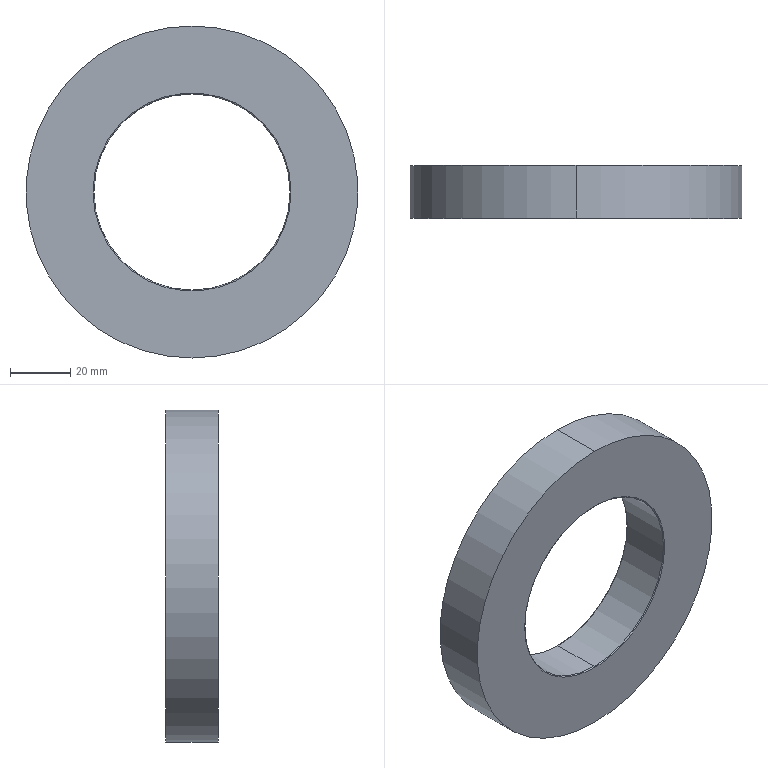Part | SolidWorks | features BaseBody 1 | 1 solid | 10 faces | box 110 x 17.5 x 110 mm | volume 108230 mm3 | cylinder 4 | torus 4 | plane 2 | commonest cylinder face diameters 65 x2 110 x2
STEP:
#1=CARTESIAN_POINT('',(-2100.15,726.569,-1577.624));
#2=VERTEX_POINT('',#1);
#3=CARTESIAN_POINT('',(-2165.75,726.569,-1577.624));
#4=VERTEX_POINT('',#3);
#5=CARTESIAN_POINT('',(-2132.95,726.569,-1577.624));
#6=DIRECTION('',(0.,-1.,0.));
#7=DIRECTION('',(0.,0.,1.));
#8=AXIS2_PLACEMENT_3D('',#5,#6,#7);
#9=CIRCLE('',#8,32.8);
#10=EDGE_CURVE('',#2,#4,#9,.T.);
#11=ORIENTED_EDGE('',*,*,#10,.F.);
#12=CARTESIAN_POINT('',(-2132.95,726.569,-1577.624));
#13=DIRECTION('',(0.,-1.,0.));
#14=DIRECTION('',(-1.,0.,0.));
#15=AXIS2_PLACEMENT_3D('',#12,#13,#14);
#16=CIRCLE('',#15,32.8);
#17=EDGE_CURVE('',#4,#2,#16,.T.);
#18=ORIENTED_EDGE('',*,*,#17,.F.);
#19=EDGE_LOOP('',(#11,#18));
#20=FACE_BOUND('',#19,.T.);
#21=CARTESIAN_POINT('',(-2132.95,726.569,-1522.624));
#22=VERTEX_POINT('',#21);
#23=CARTESIAN_POINT('',(-2132.95,726.569,-1632.624));
#24=VERTEX_POINT('',#23);
#25=CARTESIAN_POINT('',(-2132.95,726.569,-1577.624));
#26=DIRECTION('',(0.,-1.,0.));
#27=DIRECTION('',(0.,0.,1.));
#28=AXIS2_PLACEMENT_3D('',#25,#26,#27);
#29=CIRCLE('',#28,55.);
#30=EDGE_CURVE('',#22,#24,#29,.T.);
#31=ORIENTED_EDGE('',*,*,#30,.T.);
#32=CARTESIAN_POINT('',(-2132.95,726.569,-1577.624));
#33=DIRECTION('',(0.,-1.,0.));
#34=DIRECTION('',(0.,0.,-1.));
#35=AXIS2_PLACEMENT_3D('',#32,#33,#34);
#36=CIRCLE('',#35,55.);
#37=EDGE_CURVE('',#24,#22,#36,.T.);
#38=ORIENTED_EDGE('',*,*,#37,.T.);
#39=EDGE_LOOP('',(#31,#38));
#40=FACE_OUTER_BOUND('',#39,.T.);
#41=CARTESIAN_POINT('',(-2072.49,726.569,-1638.124));
#42=DIRECTION('',(0.,-1.,0.));
#43=DIRECTION('',(0.,0.,-1.));
#44=AXIS2_PLACEMENT_3D('',#41,#42,#43);
#45=PLANE('',#44);
#46=ADVANCED_FACE('',(#20,#40),#45,.T.);
#47=CARTESIAN_POINT('',(-2132.95,744.069,-1522.624));
#48=VERTEX_POINT('',#47);
#49=CARTESIAN_POINT('',(-2132.95,744.069,-1522.624));
#50=DIRECTION('',(0.,-1.,0.));
#51=VECTOR('',#50,1000.);
#52=LINE('',#49,#51);
#53=EDGE_CURVE('',#48,#22,#52,.T.);
#54=ORIENTED_EDGE('',*,*,#53,.T.);
#55=ORIENTED_EDGE('',*,*,#37,.F.);
#56=CARTESIAN_POINT('',(-2132.95,744.069,-1632.624));
#57=VERTEX_POINT('',#56);
#58=CARTESIAN_POINT('',(-2132.95,726.569,-1632.624));
#59=DIRECTION('',(0.,1.,0.));
#60=VECTOR('',#59,1000.);
#61=LINE('',#58,#60);
#62=EDGE_CURVE('',#24,#57,#61,.T.);
#63=ORIENTED_EDGE('',*,*,#62,.T.);
#64=CARTESIAN_POINT('',(-2132.95,744.069,-1577.624));
#65=DIRECTION('',(0.,1.,0.));
#66=DIRECTION('',(0.,0.,1.));
#67=AXIS2_PLACEMENT_3D('',#64,#65,#66);
#68=CIRCLE('',#67,55.);
#69=EDGE_CURVE('',#48,#57,#68,.T.);
#70=ORIENTED_EDGE('',*,*,#69,.F.);
#71=EDGE_LOOP('',(#54,#55,#63,#70));
#72=FACE_OUTER_BOUND('',#71,.T.);
#73=CARTESIAN_POINT('',(-2132.95,744.944,-1577.624));
#74=DIRECTION('',(0.,1.,0.));
#75=DIRECTION('',(-0.08716,0.,0.9962));
#76=AXIS2_PLACEMENT_3D('',#73,#74,#75);
#77=CYLINDRICAL_SURFACE('',#76,55.);
#78=ADVANCED_FACE('',(#72),#77,.T.);
#79=CARTESIAN_POINT('',(-2165.75,744.069,-1577.624));
#80=VERTEX_POINT('',#79);
#81=CARTESIAN_POINT('',(-2100.15,744.069,-1577.624));
#82=VERTEX_POINT('',#81);
#83=CARTESIAN_POINT('',(-2132.95,744.069,-1577.624));
#84=DIRECTION('',(0.,1.,0.));
#85=DIRECTION('',(-1.,0.,0.));
#86=AXIS2_PLACEMENT_3D('',#83,#84,#85);
#87=CIRCLE('',#86,32.8);
#88=EDGE_CURVE('',#80,#82,#87,.T.);
#89=ORIENTED_EDGE('',*,*,#88,.F.);
#90=CARTESIAN_POINT('',(-2132.95,744.069,-1577.624));
#91=DIRECTION('',(0.,1.,0.));
#92=DIRECTION('',(1.,0.,0.));
#93=AXIS2_PLACEMENT_3D('',#90,#91,#92);
#94=CIRCLE('',#93,32.8);
#95=EDGE_CURVE('',#82,#80,#94,.T.);
#96=ORIENTED_EDGE('',*,*,#95,.F.);
#97=EDGE_LOOP('',(#89,#96));
#98=FACE_BOUND('',#97,.T.);
#99=CARTESIAN_POINT('',(-2132.95,744.069,-1577.624));
#100=DIRECTION('',(0.,1.,0.));
#101=DIRECTION('',(0.,0.,-1.));
#102=AXIS2_PLACEMENT_3D('',#99,#100,#101);
#103=CIRCLE('',#102,55.);
#104=EDGE_CURVE('',#57,#48,#103,.T.);
#105=ORIENTED_EDGE('',*,*,#104,.T.);
#106=ORIENTED_EDGE('',*,*,#69,.T.);
#107=EDGE_LOOP('',(#105,#106));
#108=FACE_OUTER_BOUND('',#107,.T.);
#109=CARTESIAN_POINT('',(-2072.49,744.069,-1517.124));
#110=DIRECTION('',(0.,1.,0.));
#111=DIRECTION('',(1.,0.,0.));
#112=AXIS2_PLACEMENT_3D('',#109,#110,#111);
#113=PLANE('',#112);
#114=ADVANCED_FACE('',(#98,#108),#113,.T.);
#115=CARTESIAN_POINT('',(-2100.45,743.769,-1577.624));
#116=VERTEX_POINT('',#115);
#117=CARTESIAN_POINT('',(-2100.15,743.769,-1577.624));
#118=DIRECTION('',(0.,0.,-1.));
#119=DIRECTION('',(-1.,0.,0.));
#120=AXIS2_PLACEMENT_3D('',#117,#118,#119);
#121=CIRCLE('',#120,0.3);
#122=EDGE_CURVE('',#116,#82,#121,.T.);
#123=ORIENTED_EDGE('',*,*,#122,.T.);
#124=ORIENTED_EDGE('',*,*,#95,.T.);
#125=CARTESIAN_POINT('',(-2165.45,743.769,-1577.624));
#126=VERTEX_POINT('',#125);
#127=CARTESIAN_POINT('',(-2165.75,743.769,-1577.624));
#128=DIRECTION('',(0.,0.,-1.));
#129=DIRECTION('',(0.,1.,0.));
#130=AXIS2_PLACEMENT_3D('',#127,#128,#129);
#131=CIRCLE('',#130,0.3);
#132=EDGE_CURVE('',#80,#126,#131,.T.);
#133=ORIENTED_EDGE('',*,*,#132,.T.);
#134=CARTESIAN_POINT('',(-2132.95,743.769,-1610.124));
#135=VERTEX_POINT('',#134);
#136=CARTESIAN_POINT('',(-2132.95,743.769,-1577.624));
#137=DIRECTION('',(0.,-1.,0.));
#138=DIRECTION('',(-1.,0.,0.));
#139=AXIS2_PLACEMENT_3D('',#136,#137,#138);
#140=CIRCLE('',#139,32.5);
#141=EDGE_CURVE('',#126,#135,#140,.T.);
#142=ORIENTED_EDGE('',*,*,#141,.T.);
#143=CARTESIAN_POINT('',(-2132.95,743.769,-1577.624));
#144=DIRECTION('',(0.,-1.,0.));
#145=DIRECTION('',(0.,0.,-1.));
#146=AXIS2_PLACEMENT_3D('',#143,#144,#145);
#147=CIRCLE('',#146,32.5);
#148=EDGE_CURVE('',#135,#116,#147,.T.);
#149=ORIENTED_EDGE('',*,*,#148,.T.);
#150=EDGE_LOOP('',(#123,#124,#133,#142,#149));
#151=FACE_OUTER_BOUND('',#150,.T.);
#152=CARTESIAN_POINT('',(-2132.95,743.769,-1577.624));
#153=DIRECTION('',(0.,-1.,0.));
#154=DIRECTION('',(-0.9962,0.,0.08716));
#155=AXIS2_PLACEMENT_3D('',#152,#153,#154);
#156=TOROIDAL_SURFACE('',#155,32.8,0.3);
#157=ADVANCED_FACE('',(#151),#156,.T.);
#158=CARTESIAN_POINT('',(-2132.95,743.769,-1545.124));
#159=VERTEX_POINT('',#158);
#160=CARTESIAN_POINT('',(-2132.95,726.869,-1545.124));
#161=VERTEX_POINT('',#160);
#162=CARTESIAN_POINT('',(-2132.95,743.769,-1545.124));
#163=DIRECTION('',(0.,-1.,0.));
#164=VECTOR('',#163,1000.);
#165=LINE('',#162,#164);
#166=EDGE_CURVE('',#159,#161,#165,.T.);
#167=ORIENTED_EDGE('',*,*,#166,.T.);
#168=CARTESIAN_POINT('',(-2165.45,726.869,-1577.624));
#169=VERTEX_POINT('',#168);
#170=CARTESIAN_POINT('',(-2132.95,726.869,-1577.624));
#171=DIRECTION('',(0.,-1.,0.));
#172=DIRECTION('',(0.,0.,1.));
#173=AXIS2_PLACEMENT_3D('',#170,#171,#172);
#174=CIRCLE('',#173,32.5);
#175=EDGE_CURVE('',#161,#169,#174,.T.);
#176=ORIENTED_EDGE('',*,*,#175,.T.);
#177=CARTESIAN_POINT('',(-2132.95,726.869,-1610.124));
#178=VERTEX_POINT('',#177);
#179=CARTESIAN_POINT('',(-2132.95,726.869,-1577.624));
#180=DIRECTION('',(0.,-1.,0.));
#181=DIRECTION('',(-1.,0.,0.));
#182=AXIS2_PLACEMENT_3D('',#179,#180,#181);
#183=CIRCLE('',#182,32.5);
#184=EDGE_CURVE('',#169,#178,#183,.T.);
#185=ORIENTED_EDGE('',*,*,#184,.T.);
#186=CARTESIAN_POINT('',(-2132.95,726.869,-1610.124));
#187=DIRECTION('',(0.,1.,0.));
#188=VECTOR('',#187,1000.);
#189=LINE('',#186,#188);
#190=EDGE_CURVE('',#178,#135,#189,.T.);
#191=ORIENTED_EDGE('',*,*,#190,.T.);
#192=ORIENTED_EDGE('',*,*,#141,.F.);
#193=CARTESIAN_POINT('',(-2132.95,743.769,-1577.624));
#194=DIRECTION('',(0.,-1.,0.));
#195=DIRECTION('',(0.,0.,1.));
#196=AXIS2_PLACEMENT_3D('',#193,#194,#195);
#197=CIRCLE('',#196,32.5);
#198=EDGE_CURVE('',#159,#126,#197,.T.);
#199=ORIENTED_EDGE('',*,*,#198,.F.);
#200=EDGE_LOOP('',(#167,#176,#185,#191,#192,#199));
#201=FACE_OUTER_BOUND('',#200,.T.);
#202=CARTESIAN_POINT('',(-2132.95,726.024,-1577.624));
#203=DIRECTION('',(0.,1.,0.));
#204=DIRECTION('',(0.08716,0.,-0.9962));
#205=AXIS2_PLACEMENT_3D('',#202,#203,#204);
#206=CYLINDRICAL_SURFACE('',#205,32.5);
#207=ADVANCED_FACE('',(#201),#206,.F.);
#208=CARTESIAN_POINT('',(-2100.45,726.869,-1577.624));
#209=VERTEX_POINT('',#208);
#210=CARTESIAN_POINT('',(-2100.15,726.869,-1577.624));
#211=DIRECTION('',(0.,0.,-1.));
#212=DIRECTION('',(0.,-1.,0.));
#213=AXIS2_PLACEMENT_3D('',#210,#211,#212);
#214=CIRCLE('',#213,0.3);
#215=EDGE_CURVE('',#2,#209,#214,.T.);
#216=ORIENTED_EDGE('',*,*,#215,.T.);
#217=CARTESIAN_POINT('',(-2132.95,726.869,-1577.624));
#218=DIRECTION('',(0.,-1.,0.));
#219=DIRECTION('',(0.,0.,-1.));
#220=AXIS2_PLACEMENT_3D('',#217,#218,#219);
#221=CIRCLE('',#220,32.5);
#222=EDGE_CURVE('',#178,#209,#221,.T.);
#223=ORIENTED_EDGE('',*,*,#222,.F.);
#224=ORIENTED_EDGE('',*,*,#184,.F.);
#225=CARTESIAN_POINT('',(-2165.75,726.869,-1577.624));
#226=DIRECTION('',(0.,0.,-1.));
#227=DIRECTION('',(1.,0.,0.));
#228=AXIS2_PLACEMENT_3D('',#225,#226,#227);
#229=CIRCLE('',#228,0.3);
#230=EDGE_CURVE('',#169,#4,#229,.T.);
#231=ORIENTED_EDGE('',*,*,#230,.T.);
#232=ORIENTED_EDGE('',*,*,#17,.T.);
#233=EDGE_LOOP('',(#216,#223,#224,#231,#232));
#234=FACE_OUTER_BOUND('',#233,.T.);
#235=CARTESIAN_POINT('',(-2132.95,726.869,-1577.624));
#236=DIRECTION('',(0.,-1.,0.));
#237=DIRECTION('',(-0.9962,0.,0.08716));
#238=AXIS2_PLACEMENT_3D('',#235,#236,#237);
#239=TOROIDAL_SURFACE('',#238,32.8,0.3);
#240=ADVANCED_FACE('',(#234),#239,.T.);
#241=ORIENTED_EDGE('',*,*,#215,.F.);
#242=ORIENTED_EDGE('',*,*,#10,.T.);
#243=ORIENTED_EDGE('',*,*,#230,.F.);
#244=ORIENTED_EDGE('',*,*,#175,.F.);
#245=CARTESIAN_POINT('',(-2132.95,726.869,-1577.624));
#246=DIRECTION('',(0.,-1.,0.));
#247=DIRECTION('',(1.,0.,0.));
#248=AXIS2_PLACEMENT_3D('',#245,#246,#247);
#249=CIRCLE('',#248,32.5);
#250=EDGE_CURVE('',#209,#161,#249,.T.);
#251=ORIENTED_EDGE('',*,*,#250,.F.);
#252=EDGE_LOOP('',(#241,#242,#243,#244,#251));
#253=FACE_OUTER_BOUND('',#252,.T.);
#254=CARTESIAN_POINT('',(-2132.95,726.869,-1577.624));
#255=DIRECTION('',(0.,-1.,0.));
#256=DIRECTION('',(0.9962,0.,-0.08716));
#257=AXIS2_PLACEMENT_3D('',#254,#255,#256);
#258=TOROIDAL_SURFACE('',#257,32.8,0.3);
#259=ADVANCED_FACE('',(#253),#258,.T.);
#260=ORIENTED_EDGE('',*,*,#166,.F.);
#261=CARTESIAN_POINT('',(-2132.95,743.769,-1577.624));
#262=DIRECTION('',(0.,-1.,0.));
#263=DIRECTION('',(1.,0.,0.));
#264=AXIS2_PLACEMENT_3D('',#261,#262,#263);
#265=CIRCLE('',#264,32.5);
#266=EDGE_CURVE('',#116,#159,#265,.T.);
#267=ORIENTED_EDGE('',*,*,#266,.F.);
#268=ORIENTED_EDGE('',*,*,#148,.F.);
#269=ORIENTED_EDGE('',*,*,#190,.F.);
#270=ORIENTED_EDGE('',*,*,#222,.T.);
#271=ORIENTED_EDGE('',*,*,#250,.T.);
#272=EDGE_LOOP('',(#260,#267,#268,#269,#270,#271));
#273=FACE_OUTER_BOUND('',#272,.T.);
#274=CARTESIAN_POINT('',(-2132.95,726.024,-1577.624));
#275=DIRECTION('',(0.,1.,0.));
#276=DIRECTION('',(-0.08716,0.,0.9962));
#277=AXIS2_PLACEMENT_3D('',#274,#275,#276);
#278=CYLINDRICAL_SURFACE('',#277,32.5);
#279=ADVANCED_FACE('',(#273),#278,.F.);
#280=ORIENTED_EDGE('',*,*,#122,.F.);
#281=ORIENTED_EDGE('',*,*,#266,.T.);
#282=ORIENTED_EDGE('',*,*,#198,.T.);
#283=ORIENTED_EDGE('',*,*,#132,.F.);
#284=ORIENTED_EDGE('',*,*,#88,.T.);
#285=EDGE_LOOP('',(#280,#281,#282,#283,#284));
#286=FACE_OUTER_BOUND('',#285,.T.);
#287=CARTESIAN_POINT('',(-2132.95,743.769,-1577.624));
#288=DIRECTION('',(0.,-1.,0.));
#289=DIRECTION('',(0.9962,0.,-0.08716));
#290=AXIS2_PLACEMENT_3D('',#287,#288,#289);
#291=TOROIDAL_SURFACE('',#290,32.8,0.3);
#292=ADVANCED_FACE('',(#286),#291,.T.);
#293=ORIENTED_EDGE('',*,*,#53,.F.);
#294=ORIENTED_EDGE('',*,*,#104,.F.);
#295=ORIENTED_EDGE('',*,*,#62,.F.);
#296=ORIENTED_EDGE('',*,*,#30,.F.);
#297=EDGE_LOOP('',(#293,#294,#295,#296));
#298=FACE_OUTER_BOUND('',#297,.T.);
#299=CARTESIAN_POINT('',(-2132.95,744.944,-1577.624));
#300=DIRECTION('',(0.,1.,0.));
#301=DIRECTION('',(0.08716,0.,-0.9962));
#302=AXIS2_PLACEMENT_3D('',#299,#300,#301);
#303=CYLINDRICAL_SURFACE('',#302,55.);
#304=ADVANCED_FACE('',(#298),#303,.T.);
#305=CLOSED_SHELL('',(#46,#78,#114,#157,#207,#240,#259,#279,#292,#304));
#306=MANIFOLD_SOLID_BREP('',#305);
#307=CARTESIAN_POINT('',(0.,0.,0.));
#308=DIRECTION('',(0.,0.,1.));
#309=DIRECTION('',(1.,0.,0.));
#310=AXIS2_PLACEMENT_3D('',#307,#308,#309);
#311=(LENGTH_UNIT()NAMED_UNIT(*)SI_UNIT(.MILLI.,.METRE.));
#312=UNCERTAINTY_MEASURE_WITH_UNIT(LENGTH_MEASURE(0.00001),#311,'','');
#313=(NAMED_UNIT(*)PLANE_ANGLE_UNIT()SI_UNIT($,.RADIAN.));
#314=(NAMED_UNIT(*)SI_UNIT($,.STERADIAN.)SOLID_ANGLE_UNIT());
#315=(GEOMETRIC_REPRESENTATION_CONTEXT(3)GLOBAL_UNCERTAINTY_ASSIGNED_CONTEXT((#312))GLOBAL_UNIT_ASSIGNED_CONTEXT((#311,#313,#314))REPRESENTATION_CONTEXT('',''));
#316=ADVANCED_BREP_SHAPE_REPRESENTATION('',(#306,#310),#315);